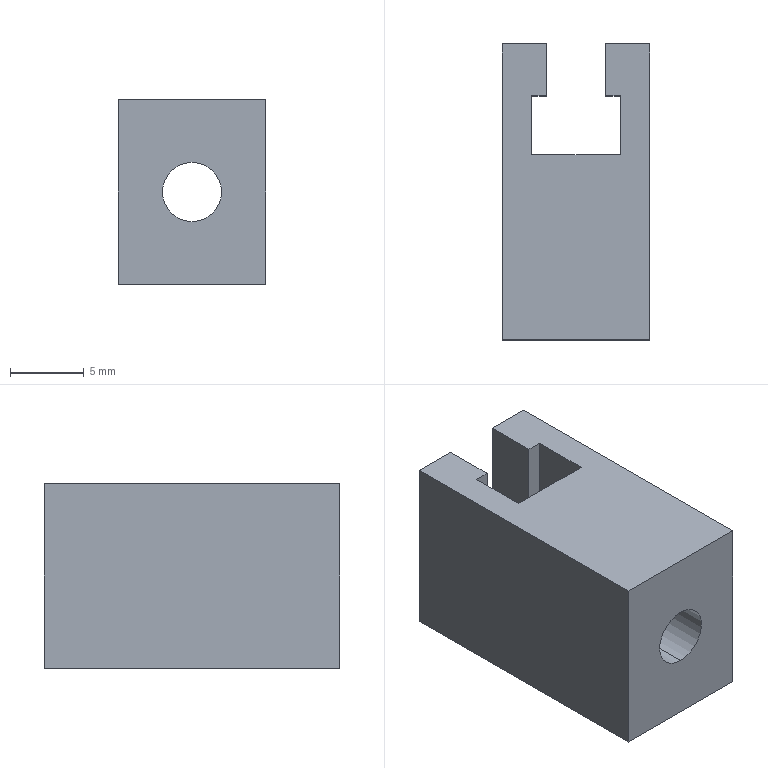Part | STEP file | 1 solid | 16 faces | box 10 x 20 x 12.5 mm | volume 1868 mm3 | plane 14 | cylinder 2 | commonest cylinder face diameters 4 x2
STEP:
#1=CARTESIAN_POINT('',(0.,0.,0.));
#2=DIRECTION('',(0.,0.,1.));
#3=DIRECTION('',(1.,0.,0.));
#4=AXIS2_PLACEMENT_3D('',#1,#2,#3);
#5=CARTESIAN_POINT('',(-38.279,-90.,99.036));
#6=VERTEX_POINT('',#5);
#7=CARTESIAN_POINT('',(-38.279,-77.5,99.036));
#8=VERTEX_POINT('',#7);
#9=CARTESIAN_POINT('',(-38.279,-90.,99.036));
#10=DIRECTION('',(0.,1.,0.));
#11=VECTOR('',#10,1.);
#12=LINE('',#9,#11);
#13=CARTESIAN_POINT('',(-38.279,-90.,97.036));
#14=DIRECTION('',(0.,1.,0.));
#15=DIRECTION('',(0.,0.,1.));
#16=AXIS2_PLACEMENT_3D('',#13,#14,#15);
#17=CYLINDRICAL_SURFACE('',#16,2.);
#18=CARTESIAN_POINT('',(6.283,0.));
#19=DIRECTION('',(0.,1.));
#20=VECTOR('',#19,1.);
#21=LINE('',#18,#20);
#22=(GEOMETRIC_REPRESENTATION_CONTEXT(2)PARAMETRIC_REPRESENTATION_CONTEXT()REPRESENTATION_CONTEXT('',''));
#23=DEFINITIONAL_REPRESENTATION('',(#21),#22);
#24=PCURVE('',#17,#23);
#25=CARTESIAN_POINT('',(-38.279,-90.,97.036));
#26=DIRECTION('',(0.,1.,0.));
#27=DIRECTION('',(0.,0.,1.));
#28=AXIS2_PLACEMENT_3D('',#25,#26,#27);
#29=CYLINDRICAL_SURFACE('',#28,2.);
#30=CARTESIAN_POINT('',(0.,0.));
#31=DIRECTION('',(0.,1.));
#32=VECTOR('',#31,1.);
#33=LINE('',#30,#32);
#34=(GEOMETRIC_REPRESENTATION_CONTEXT(2)PARAMETRIC_REPRESENTATION_CONTEXT()REPRESENTATION_CONTEXT('',''));
#35=DEFINITIONAL_REPRESENTATION('',(#33),#34);
#36=PCURVE('',#29,#35);
#37=SURFACE_CURVE('',#12,(#24,#36),.PCURVE_S1.);
#38=EDGE_CURVE('',#6,#8,#37,.T.);
#39=ORIENTED_EDGE('',*,*,#38,.T.);
#40=CARTESIAN_POINT('',(-38.279,-77.5,95.036));
#41=VERTEX_POINT('',#40);
#42=CARTESIAN_POINT('',(-38.279,-77.5,97.036));
#43=DIRECTION('',(0.,-1.,0.));
#44=DIRECTION('',(0.,0.,-1.));
#45=AXIS2_PLACEMENT_3D('',#42,#43,#44);
#46=CIRCLE('',#45,2.);
#47=CARTESIAN_POINT('',(9.425,12.5));
#48=DIRECTION('',(-1.,0.));
#49=VECTOR('',#48,1.);
#50=LINE('',#47,#49);
#51=(GEOMETRIC_REPRESENTATION_CONTEXT(2)PARAMETRIC_REPRESENTATION_CONTEXT()REPRESENTATION_CONTEXT('',''));
#52=DEFINITIONAL_REPRESENTATION('',(#50),#51);
#53=PCURVE('',#17,#52);
#54=CARTESIAN_POINT('',(-72.862,-77.5,115.03));
#55=DIRECTION('',(0.,-1.,0.));
#56=DIRECTION('',(0.,0.,-1.));
#57=AXIS2_PLACEMENT_3D('',#54,#55,#56);
#58=PLANE('',#57);
#59=CARTESIAN_POINT('',(17.994,34.584));
#60=DIRECTION('',(1.,0.));
#61=AXIS2_PLACEMENT_2D('',#59,#60);
#62=CIRCLE('',#61,2.);
#63=(GEOMETRIC_REPRESENTATION_CONTEXT(2)PARAMETRIC_REPRESENTATION_CONTEXT()REPRESENTATION_CONTEXT('',''));
#64=DEFINITIONAL_REPRESENTATION('',(#62),#63);
#65=PCURVE('',#58,#64);
#66=SURFACE_CURVE('',#46,(#53,#65),.PCURVE_S1.);
#67=EDGE_CURVE('',#8,#41,#66,.T.);
#68=ORIENTED_EDGE('',*,*,#67,.T.);
#69=CARTESIAN_POINT('',(-38.279,-90.,95.036));
#70=VERTEX_POINT('',#69);
#71=CARTESIAN_POINT('',(-38.279,-90.,95.036));
#72=DIRECTION('',(0.,1.,0.));
#73=VECTOR('',#72,1.);
#74=LINE('',#71,#73);
#75=CARTESIAN_POINT('',(3.142,0.));
#76=DIRECTION('',(0.,1.));
#77=VECTOR('',#76,1.);
#78=LINE('',#75,#77);
#79=(GEOMETRIC_REPRESENTATION_CONTEXT(2)PARAMETRIC_REPRESENTATION_CONTEXT()REPRESENTATION_CONTEXT('',''));
#80=DEFINITIONAL_REPRESENTATION('',(#78),#79);
#81=PCURVE('',#17,#80);
#82=CARTESIAN_POINT('',(3.142,0.));
#83=DIRECTION('',(0.,1.));
#84=VECTOR('',#83,1.);
#85=LINE('',#82,#84);
#86=(GEOMETRIC_REPRESENTATION_CONTEXT(2)PARAMETRIC_REPRESENTATION_CONTEXT()REPRESENTATION_CONTEXT('',''));
#87=DEFINITIONAL_REPRESENTATION('',(#85),#86);
#88=PCURVE('',#29,#87);
#89=SURFACE_CURVE('',#74,(#81,#88),.PCURVE_S1.);
#90=EDGE_CURVE('',#70,#41,#89,.T.);
#91=ORIENTED_EDGE('',*,*,#90,.F.);
#92=CARTESIAN_POINT('',(-38.279,-90.,97.036));
#93=DIRECTION('',(0.,1.,0.));
#94=DIRECTION('',(0.,0.,1.));
#95=AXIS2_PLACEMENT_3D('',#92,#93,#94);
#96=CIRCLE('',#95,2.);
#97=CARTESIAN_POINT('',(0.,0.));
#98=DIRECTION('',(1.,0.));
#99=VECTOR('',#98,1.);
#100=LINE('',#97,#99);
#101=(GEOMETRIC_REPRESENTATION_CONTEXT(2)PARAMETRIC_REPRESENTATION_CONTEXT()REPRESENTATION_CONTEXT('',''));
#102=DEFINITIONAL_REPRESENTATION('',(#100),#101);
#103=PCURVE('',#17,#102);
#104=CARTESIAN_POINT('',(-38.279,-90.,90.286));
#105=DIRECTION('',(0.,-1.,0.));
#106=DIRECTION('',(0.,0.,-1.));
#107=AXIS2_PLACEMENT_3D('',#104,#105,#106);
#108=PLANE('',#107);
#109=CARTESIAN_POINT('',(-8.75,0.));
#110=CARTESIAN_POINT('',(-8.75,3.464));
#111=CARTESIAN_POINT('',(-5.75,1.732));
#112=CARTESIAN_POINT('',(-2.75,0.));
#113=CARTESIAN_POINT('',(-5.75,-1.732));
#114=CARTESIAN_POINT('',(-8.75,-3.464));
#115=CARTESIAN_POINT('',(-8.75,0.));
#116=(BOUNDED_CURVE()B_SPLINE_CURVE(2,(#109,#110,#111,#112,#113,#114,#115),.UNSPECIFIED.,.T.,.F.)B_SPLINE_CURVE_WITH_KNOTS((1,2,2,2,2,1),(-2.094,0.,2.094,4.189,6.283,8.378),.UNSPECIFIED.)CURVE()GEOMETRIC_REPRESENTATION_ITEM()RATIONAL_B_SPLINE_CURVE((1.,0.5,1.,0.5,1.,0.5,1.))REPRESENTATION_ITEM(''));
#117=(GEOMETRIC_REPRESENTATION_CONTEXT(2)PARAMETRIC_REPRESENTATION_CONTEXT()REPRESENTATION_CONTEXT('',''));
#118=DEFINITIONAL_REPRESENTATION('',(#116),#117);
#119=PCURVE('',#108,#118);
#120=SURFACE_CURVE('',#96,(#103,#119),.PCURVE_S1.);
#121=EDGE_CURVE('',#70,#6,#120,.T.);
#122=ORIENTED_EDGE('',*,*,#121,.T.);
#123=EDGE_LOOP('',(#39,#68,#91,#122));
#124=FACE_BOUND('',#123,.F.);
#125=ADVANCED_FACE('',(#124),#17,.F.);
#126=CARTESIAN_POINT('',(-41.279,-73.5,103.286));
#127=VERTEX_POINT('',#126);
#128=CARTESIAN_POINT('',(-40.279,-73.5,103.286));
#129=VERTEX_POINT('',#128);
#130=CARTESIAN_POINT('',(-38.279,-73.5,103.286));
#131=DIRECTION('',(1.,0.,0.));
#132=VECTOR('',#131,1.);
#133=LINE('',#130,#132);
#134=CARTESIAN_POINT('',(-38.279,-85.,103.286));
#135=DIRECTION('',(0.,0.,1.));
#136=DIRECTION('',(1.,0.,0.));
#137=AXIS2_PLACEMENT_3D('',#134,#135,#136);
#138=PLANE('',#137);
#139=CARTESIAN_POINT('',(0.,11.5));
#140=DIRECTION('',(1.,0.));
#141=VECTOR('',#140,1.);
#142=LINE('',#139,#141);
#143=(GEOMETRIC_REPRESENTATION_CONTEXT(2)PARAMETRIC_REPRESENTATION_CONTEXT()REPRESENTATION_CONTEXT('',''));
#144=DEFINITIONAL_REPRESENTATION('',(#142),#143);
#145=PCURVE('',#138,#144);
#146=CARTESIAN_POINT('',(-38.279,-73.5,95.192));
#147=DIRECTION('',(0.,-1.,0.));
#148=DIRECTION('',(0.,0.,-1.));
#149=AXIS2_PLACEMENT_3D('',#146,#147,#148);
#150=PLANE('',#149);
#151=CARTESIAN_POINT('',(-8.093,0.));
#152=DIRECTION('',(0.,1.));
#153=VECTOR('',#152,1.);
#154=LINE('',#151,#153);
#155=(GEOMETRIC_REPRESENTATION_CONTEXT(2)PARAMETRIC_REPRESENTATION_CONTEXT()REPRESENTATION_CONTEXT('',''));
#156=DEFINITIONAL_REPRESENTATION('',(#154),#155);
#157=PCURVE('',#150,#156);
#158=SURFACE_CURVE('',#133,(#145,#157),.PCURVE_S1.);
#159=EDGE_CURVE('',#127,#129,#158,.T.);
#160=ORIENTED_EDGE('',*,*,#159,.T.);
#161=CARTESIAN_POINT('',(-40.279,-70.,103.286));
#162=VERTEX_POINT('',#161);
#163=CARTESIAN_POINT('',(-40.279,-85.,103.286));
#164=DIRECTION('',(0.,1.,0.));
#165=VECTOR('',#164,1.);
#166=LINE('',#163,#165);
#167=CARTESIAN_POINT('',(-2.,0.));
#168=DIRECTION('',(0.,1.));
#169=VECTOR('',#168,1.);
#170=LINE('',#167,#169);
#171=(GEOMETRIC_REPRESENTATION_CONTEXT(2)PARAMETRIC_REPRESENTATION_CONTEXT()REPRESENTATION_CONTEXT('',''));
#172=DEFINITIONAL_REPRESENTATION('',(#170),#171);
#173=PCURVE('',#138,#172);
#174=CARTESIAN_POINT('',(-40.279,-38.669,100.65));
#175=DIRECTION('',(1.,0.,0.));
#176=DIRECTION('',(0.,0.,-1.));
#177=AXIS2_PLACEMENT_3D('',#174,#175,#176);
#178=PLANE('',#177);
#179=CARTESIAN_POINT('',(-2.636,-46.331));
#180=DIRECTION('',(0.,1.));
#181=VECTOR('',#180,1.);
#182=LINE('',#179,#181);
#183=(GEOMETRIC_REPRESENTATION_CONTEXT(2)PARAMETRIC_REPRESENTATION_CONTEXT()REPRESENTATION_CONTEXT('',''));
#184=DEFINITIONAL_REPRESENTATION('',(#182),#183);
#185=PCURVE('',#178,#184);
#186=SURFACE_CURVE('',#166,(#173,#185),.PCURVE_S1.);
#187=EDGE_CURVE('',#129,#162,#186,.T.);
#188=ORIENTED_EDGE('',*,*,#187,.T.);
#189=CARTESIAN_POINT('',(-43.279,-70.,103.286));
#190=VERTEX_POINT('',#189);
#191=CARTESIAN_POINT('',(-38.279,-70.,103.286));
#192=DIRECTION('',(1.,0.,0.));
#193=VECTOR('',#192,1.);
#194=LINE('',#191,#193);
#195=CARTESIAN_POINT('',(0.,15.));
#196=DIRECTION('',(1.,0.));
#197=VECTOR('',#196,1.);
#198=LINE('',#195,#197);
#199=(GEOMETRIC_REPRESENTATION_CONTEXT(2)PARAMETRIC_REPRESENTATION_CONTEXT()REPRESENTATION_CONTEXT('',''));
#200=DEFINITIONAL_REPRESENTATION('',(#198),#199);
#201=PCURVE('',#138,#200);
#202=CARTESIAN_POINT('',(-38.279,-70.,90.286));
#203=DIRECTION('',(0.,1.,0.));
#204=DIRECTION('',(0.,0.,1.));
#205=AXIS2_PLACEMENT_3D('',#202,#203,#204);
#206=PLANE('',#205);
#207=CARTESIAN_POINT('',(13.,0.));
#208=DIRECTION('',(0.,1.));
#209=VECTOR('',#208,1.);
#210=LINE('',#207,#209);
#211=(GEOMETRIC_REPRESENTATION_CONTEXT(2)PARAMETRIC_REPRESENTATION_CONTEXT()REPRESENTATION_CONTEXT('',''));
#212=DEFINITIONAL_REPRESENTATION('',(#210),#211);
#213=PCURVE('',#206,#212);
#214=SURFACE_CURVE('',#194,(#201,#213),.PCURVE_S1.);
#215=EDGE_CURVE('',#190,#162,#214,.T.);
#216=ORIENTED_EDGE('',*,*,#215,.F.);
#217=CARTESIAN_POINT('',(-43.279,-90.,103.286));
#218=VERTEX_POINT('',#217);
#219=CARTESIAN_POINT('',(-43.279,-85.,103.286));
#220=DIRECTION('',(0.,1.,0.));
#221=VECTOR('',#220,1.);
#222=LINE('',#219,#221);
#223=CARTESIAN_POINT('',(-5.,0.));
#224=DIRECTION('',(0.,1.));
#225=VECTOR('',#224,1.);
#226=LINE('',#223,#225);
#227=(GEOMETRIC_REPRESENTATION_CONTEXT(2)PARAMETRIC_REPRESENTATION_CONTEXT()REPRESENTATION_CONTEXT('',''));
#228=DEFINITIONAL_REPRESENTATION('',(#226),#227);
#229=PCURVE('',#138,#228);
#230=CARTESIAN_POINT('',(-43.279,-85.,90.286));
#231=DIRECTION('',(-1.,0.,0.));
#232=DIRECTION('',(0.,0.,1.));
#233=AXIS2_PLACEMENT_3D('',#230,#231,#232);
#234=PLANE('',#233);
#235=CARTESIAN_POINT('',(13.,0.));
#236=DIRECTION('',(0.,1.));
#237=VECTOR('',#236,1.);
#238=LINE('',#235,#237);
#239=(GEOMETRIC_REPRESENTATION_CONTEXT(2)PARAMETRIC_REPRESENTATION_CONTEXT()REPRESENTATION_CONTEXT('',''));
#240=DEFINITIONAL_REPRESENTATION('',(#238),#239);
#241=PCURVE('',#234,#240);
#242=SURFACE_CURVE('',#222,(#229,#241),.PCURVE_S1.);
#243=EDGE_CURVE('',#218,#190,#242,.T.);
#244=ORIENTED_EDGE('',*,*,#243,.F.);
#245=CARTESIAN_POINT('',(-33.279,-90.,103.286));
#246=VERTEX_POINT('',#245);
#247=CARTESIAN_POINT('',(-38.279,-90.,103.286));
#248=DIRECTION('',(-1.,0.,0.));
#249=VECTOR('',#248,1.);
#250=LINE('',#247,#249);
#251=CARTESIAN_POINT('',(0.,-5.));
#252=DIRECTION('',(-1.,0.));
#253=VECTOR('',#252,1.);
#254=LINE('',#251,#253);
#255=(GEOMETRIC_REPRESENTATION_CONTEXT(2)PARAMETRIC_REPRESENTATION_CONTEXT()REPRESENTATION_CONTEXT('',''));
#256=DEFINITIONAL_REPRESENTATION('',(#254),#255);
#257=PCURVE('',#138,#256);
#258=CARTESIAN_POINT('',(-13.,0.));
#259=DIRECTION('',(0.,-1.));
#260=VECTOR('',#259,1.);
#261=LINE('',#258,#260);
#262=(GEOMETRIC_REPRESENTATION_CONTEXT(2)PARAMETRIC_REPRESENTATION_CONTEXT()REPRESENTATION_CONTEXT('',''));
#263=DEFINITIONAL_REPRESENTATION('',(#261),#262);
#264=PCURVE('',#108,#263);
#265=SURFACE_CURVE('',#250,(#257,#264),.PCURVE_S1.);
#266=EDGE_CURVE('',#246,#218,#265,.T.);
#267=ORIENTED_EDGE('',*,*,#266,.F.);
#268=CARTESIAN_POINT('',(-33.279,-70.,103.286));
#269=VERTEX_POINT('',#268);
#270=CARTESIAN_POINT('',(-33.279,-85.,103.286));
#271=DIRECTION('',(0.,-1.,0.));
#272=VECTOR('',#271,1.);
#273=LINE('',#270,#272);
#274=CARTESIAN_POINT('',(5.,0.));
#275=DIRECTION('',(0.,-1.));
#276=VECTOR('',#275,1.);
#277=LINE('',#274,#276);
#278=(GEOMETRIC_REPRESENTATION_CONTEXT(2)PARAMETRIC_REPRESENTATION_CONTEXT()REPRESENTATION_CONTEXT('',''));
#279=DEFINITIONAL_REPRESENTATION('',(#277),#278);
#280=PCURVE('',#138,#279);
#281=CARTESIAN_POINT('',(-33.279,-85.,90.286));
#282=DIRECTION('',(1.,0.,0.));
#283=DIRECTION('',(0.,0.,-1.));
#284=AXIS2_PLACEMENT_3D('',#281,#282,#283);
#285=PLANE('',#284);
#286=CARTESIAN_POINT('',(-13.,0.));
#287=DIRECTION('',(0.,-1.));
#288=VECTOR('',#287,1.);
#289=LINE('',#286,#288);
#290=(GEOMETRIC_REPRESENTATION_CONTEXT(2)PARAMETRIC_REPRESENTATION_CONTEXT()REPRESENTATION_CONTEXT('',''));
#291=DEFINITIONAL_REPRESENTATION('',(#289),#290);
#292=PCURVE('',#285,#291);
#293=SURFACE_CURVE('',#273,(#280,#292),.PCURVE_S1.);
#294=EDGE_CURVE('',#269,#246,#293,.T.);
#295=ORIENTED_EDGE('',*,*,#294,.F.);
#296=CARTESIAN_POINT('',(-36.279,-70.,103.286));
#297=VERTEX_POINT('',#296);
#298=CARTESIAN_POINT('',(-38.279,-70.,103.286));
#299=DIRECTION('',(1.,0.,0.));
#300=VECTOR('',#299,1.);
#301=LINE('',#298,#300);
#302=CARTESIAN_POINT('',(0.,15.));
#303=DIRECTION('',(1.,0.));
#304=VECTOR('',#303,1.);
#305=LINE('',#302,#304);
#306=(GEOMETRIC_REPRESENTATION_CONTEXT(2)PARAMETRIC_REPRESENTATION_CONTEXT()REPRESENTATION_CONTEXT('',''));
#307=DEFINITIONAL_REPRESENTATION('',(#305),#306);
#308=PCURVE('',#138,#307);
#309=CARTESIAN_POINT('',(-38.279,-70.,90.286));
#310=DIRECTION('',(0.,1.,0.));
#311=DIRECTION('',(0.,0.,1.));
#312=AXIS2_PLACEMENT_3D('',#309,#310,#311);
#313=PLANE('',#312);
#314=CARTESIAN_POINT('',(13.,0.));
#315=DIRECTION('',(0.,1.));
#316=VECTOR('',#315,1.);
#317=LINE('',#314,#316);
#318=(GEOMETRIC_REPRESENTATION_CONTEXT(2)PARAMETRIC_REPRESENTATION_CONTEXT()REPRESENTATION_CONTEXT('',''));
#319=DEFINITIONAL_REPRESENTATION('',(#317),#318);
#320=PCURVE('',#313,#319);
#321=SURFACE_CURVE('',#301,(#308,#320),.PCURVE_S1.);
#322=EDGE_CURVE('',#297,#269,#321,.T.);
#323=ORIENTED_EDGE('',*,*,#322,.F.);
#324=CARTESIAN_POINT('',(-36.279,-73.5,103.286));
#325=VERTEX_POINT('',#324);
#326=CARTESIAN_POINT('',(-36.279,-85.,103.286));
#327=DIRECTION('',(0.,1.,0.));
#328=VECTOR('',#327,1.);
#329=LINE('',#326,#328);
#330=CARTESIAN_POINT('',(2.,0.));
#331=DIRECTION('',(0.,1.));
#332=VECTOR('',#331,1.);
#333=LINE('',#330,#332);
#334=(GEOMETRIC_REPRESENTATION_CONTEXT(2)PARAMETRIC_REPRESENTATION_CONTEXT()REPRESENTATION_CONTEXT('',''));
#335=DEFINITIONAL_REPRESENTATION('',(#333),#334);
#336=PCURVE('',#138,#335);
#337=CARTESIAN_POINT('',(-36.279,-3.669,115.562));
#338=DIRECTION('',(1.,0.,0.));
#339=DIRECTION('',(0.,0.,-1.));
#340=AXIS2_PLACEMENT_3D('',#337,#338,#339);
#341=PLANE('',#340);
#342=CARTESIAN_POINT('',(12.276,-81.331));
#343=DIRECTION('',(0.,1.));
#344=VECTOR('',#343,1.);
#345=LINE('',#342,#344);
#346=(GEOMETRIC_REPRESENTATION_CONTEXT(2)PARAMETRIC_REPRESENTATION_CONTEXT()REPRESENTATION_CONTEXT('',''));
#347=DEFINITIONAL_REPRESENTATION('',(#345),#346);
#348=PCURVE('',#341,#347);
#349=SURFACE_CURVE('',#329,(#336,#348),.PCURVE_S1.);
#350=EDGE_CURVE('',#325,#297,#349,.T.);
#351=ORIENTED_EDGE('',*,*,#350,.F.);
#352=CARTESIAN_POINT('',(-35.279,-73.5,103.286));
#353=VERTEX_POINT('',#352);
#354=CARTESIAN_POINT('',(-38.279,-73.5,103.286));
#355=DIRECTION('',(1.,0.,0.));
#356=VECTOR('',#355,1.);
#357=LINE('',#354,#356);
#358=CARTESIAN_POINT('',(0.,11.5));
#359=DIRECTION('',(1.,0.));
#360=VECTOR('',#359,1.);
#361=LINE('',#358,#360);
#362=(GEOMETRIC_REPRESENTATION_CONTEXT(2)PARAMETRIC_REPRESENTATION_CONTEXT()REPRESENTATION_CONTEXT('',''));
#363=DEFINITIONAL_REPRESENTATION('',(#361),#362);
#364=PCURVE('',#138,#363);
#365=CARTESIAN_POINT('',(-38.279,-73.5,95.192));
#366=DIRECTION('',(0.,-1.,0.));
#367=DIRECTION('',(0.,0.,-1.));
#368=AXIS2_PLACEMENT_3D('',#365,#366,#367);
#369=PLANE('',#368);
#370=CARTESIAN_POINT('',(-8.093,0.));
#371=DIRECTION('',(0.,1.));
#372=VECTOR('',#371,1.);
#373=LINE('',#370,#372);
#374=(GEOMETRIC_REPRESENTATION_CONTEXT(2)PARAMETRIC_REPRESENTATION_CONTEXT()REPRESENTATION_CONTEXT('',''));
#375=DEFINITIONAL_REPRESENTATION('',(#373),#374);
#376=PCURVE('',#369,#375);
#377=SURFACE_CURVE('',#357,(#364,#376),.PCURVE_S1.);
#378=EDGE_CURVE('',#325,#353,#377,.T.);
#379=ORIENTED_EDGE('',*,*,#378,.T.);
#380=CARTESIAN_POINT('',(-35.279,-77.5,103.286));
#381=VERTEX_POINT('',#380);
#382=CARTESIAN_POINT('',(-35.279,-85.,103.286));
#383=DIRECTION('',(0.,1.,0.));
#384=VECTOR('',#383,1.);
#385=LINE('',#382,#384);
#386=CARTESIAN_POINT('',(3.,0.));
#387=DIRECTION('',(0.,1.));
#388=VECTOR('',#387,1.);
#389=LINE('',#386,#388);
#390=(GEOMETRIC_REPRESENTATION_CONTEXT(2)PARAMETRIC_REPRESENTATION_CONTEXT()REPRESENTATION_CONTEXT('',''));
#391=DEFINITIONAL_REPRESENTATION('',(#389),#390);
#392=PCURVE('',#138,#391);
#393=CARTESIAN_POINT('',(-35.279,-3.669,115.562));
#394=DIRECTION('',(1.,0.,0.));
#395=DIRECTION('',(0.,0.,-1.));
#396=AXIS2_PLACEMENT_3D('',#393,#394,#395);
#397=PLANE('',#396);
#398=CARTESIAN_POINT('',(12.276,-81.331));
#399=DIRECTION('',(0.,1.));
#400=VECTOR('',#399,1.);
#401=LINE('',#398,#400);
#402=(GEOMETRIC_REPRESENTATION_CONTEXT(2)PARAMETRIC_REPRESENTATION_CONTEXT()REPRESENTATION_CONTEXT('',''));
#403=DEFINITIONAL_REPRESENTATION('',(#401),#402);
#404=PCURVE('',#397,#403);
#405=SURFACE_CURVE('',#385,(#392,#404),.PCURVE_S1.);
#406=EDGE_CURVE('',#381,#353,#405,.T.);
#407=ORIENTED_EDGE('',*,*,#406,.F.);
#408=CARTESIAN_POINT('',(-41.279,-77.5,103.286));
#409=VERTEX_POINT('',#408);
#410=CARTESIAN_POINT('',(-38.279,-77.5,103.286));
#411=DIRECTION('',(1.,0.,0.));
#412=VECTOR('',#411,1.);
#413=LINE('',#410,#412);
#414=CARTESIAN_POINT('',(0.,7.5));
#415=DIRECTION('',(1.,0.));
#416=VECTOR('',#415,1.);
#417=LINE('',#414,#416);
#418=(GEOMETRIC_REPRESENTATION_CONTEXT(2)PARAMETRIC_REPRESENTATION_CONTEXT()REPRESENTATION_CONTEXT('',''));
#419=DEFINITIONAL_REPRESENTATION('',(#417),#418);
#420=PCURVE('',#138,#419);
#421=CARTESIAN_POINT('',(11.744,34.584));
#422=DIRECTION('',(0.,1.));
#423=VECTOR('',#422,1.);
#424=LINE('',#421,#423);
#425=(GEOMETRIC_REPRESENTATION_CONTEXT(2)PARAMETRIC_REPRESENTATION_CONTEXT()REPRESENTATION_CONTEXT('',''));
#426=DEFINITIONAL_REPRESENTATION('',(#424),#425);
#427=PCURVE('',#58,#426);
#428=SURFACE_CURVE('',#413,(#420,#427),.PCURVE_S1.);
#429=EDGE_CURVE('',#409,#381,#428,.T.);
#430=ORIENTED_EDGE('',*,*,#429,.F.);
#431=CARTESIAN_POINT('',(-41.279,-85.,103.286));
#432=DIRECTION('',(0.,1.,0.));
#433=VECTOR('',#432,1.);
#434=LINE('',#431,#433);
#435=CARTESIAN_POINT('',(-3.,0.));
#436=DIRECTION('',(0.,1.));
#437=VECTOR('',#436,1.);
#438=LINE('',#435,#437);
#439=(GEOMETRIC_REPRESENTATION_CONTEXT(2)PARAMETRIC_REPRESENTATION_CONTEXT()REPRESENTATION_CONTEXT('',''));
#440=DEFINITIONAL_REPRESENTATION('',(#438),#439);
#441=PCURVE('',#138,#440);
#442=CARTESIAN_POINT('',(-41.279,-38.669,100.65));
#443=DIRECTION('',(1.,0.,0.));
#444=DIRECTION('',(0.,0.,-1.));
#445=AXIS2_PLACEMENT_3D('',#442,#443,#444);
#446=PLANE('',#445);
#447=CARTESIAN_POINT('',(-2.636,-46.331));
#448=DIRECTION('',(0.,1.));
#449=VECTOR('',#448,1.);
#450=LINE('',#447,#449);
#451=(GEOMETRIC_REPRESENTATION_CONTEXT(2)PARAMETRIC_REPRESENTATION_CONTEXT()REPRESENTATION_CONTEXT('',''));
#452=DEFINITIONAL_REPRESENTATION('',(#450),#451);
#453=PCURVE('',#446,#452);
#454=SURFACE_CURVE('',#434,(#441,#453),.PCURVE_S1.);
#455=EDGE_CURVE('',#409,#127,#454,.T.);
#456=ORIENTED_EDGE('',*,*,#455,.T.);
#457=EDGE_LOOP('',(#160,#188,#216,#244,#267,#295,#323,#351,#379,#407,#430,#456));
#458=FACE_BOUND('',#457,.T.);
#459=ADVANCED_FACE('',(#458),#138,.T.);
#460=ORIENTED_EDGE('',*,*,#215,.T.);
#461=CARTESIAN_POINT('',(-40.279,-70.,90.786));
#462=VERTEX_POINT('',#461);
#463=CARTESIAN_POINT('',(-40.279,-70.,90.286));
#464=DIRECTION('',(0.,0.,-1.));
#465=VECTOR('',#464,1.);
#466=LINE('',#463,#465);
#467=CARTESIAN_POINT('',(0.,-2.));
#468=DIRECTION('',(-1.,0.));
#469=VECTOR('',#468,1.);
#470=LINE('',#467,#469);
#471=(GEOMETRIC_REPRESENTATION_CONTEXT(2)PARAMETRIC_REPRESENTATION_CONTEXT()REPRESENTATION_CONTEXT('',''));
#472=DEFINITIONAL_REPRESENTATION('',(#470),#471);
#473=PCURVE('',#206,#472);
#474=CARTESIAN_POINT('',(10.364,-31.331));
#475=DIRECTION('',(1.,0.));
#476=VECTOR('',#475,1.);
#477=LINE('',#474,#476);
#478=(GEOMETRIC_REPRESENTATION_CONTEXT(2)PARAMETRIC_REPRESENTATION_CONTEXT()REPRESENTATION_CONTEXT('',''));
#479=DEFINITIONAL_REPRESENTATION('',(#477),#478);
#480=PCURVE('',#178,#479);
#481=SURFACE_CURVE('',#466,(#473,#480),.PCURVE_S1.);
#482=EDGE_CURVE('',#162,#462,#481,.T.);
#483=ORIENTED_EDGE('',*,*,#482,.T.);
#484=CARTESIAN_POINT('',(-43.279,-70.,90.786));
#485=VERTEX_POINT('',#484);
#486=CARTESIAN_POINT('',(-38.279,-70.,90.786));
#487=DIRECTION('',(-1.,0.,0.));
#488=VECTOR('',#487,1.);
#489=LINE('',#486,#488);
#490=CARTESIAN_POINT('',(0.5,0.));
#491=DIRECTION('',(0.,-1.));
#492=VECTOR('',#491,1.);
#493=LINE('',#490,#492);
#494=(GEOMETRIC_REPRESENTATION_CONTEXT(2)PARAMETRIC_REPRESENTATION_CONTEXT()REPRESENTATION_CONTEXT('',''));
#495=DEFINITIONAL_REPRESENTATION('',(#493),#494);
#496=PCURVE('',#206,#495);
#497=CARTESIAN_POINT('',(-38.279,-85.,90.786));
#498=DIRECTION('',(0.,0.,-1.));
#499=DIRECTION('',(-1.,0.,0.));
#500=AXIS2_PLACEMENT_3D('',#497,#498,#499);
#501=PLANE('',#500);
#502=CARTESIAN_POINT('',(0.,15.));
#503=DIRECTION('',(1.,0.));
#504=VECTOR('',#503,1.);
#505=LINE('',#502,#504);
#506=(GEOMETRIC_REPRESENTATION_CONTEXT(2)PARAMETRIC_REPRESENTATION_CONTEXT()REPRESENTATION_CONTEXT('',''));
#507=DEFINITIONAL_REPRESENTATION('',(#505),#506);
#508=PCURVE('',#501,#507);
#509=SURFACE_CURVE('',#489,(#496,#508),.PCURVE_S1.);
#510=EDGE_CURVE('',#462,#485,#509,.T.);
#511=ORIENTED_EDGE('',*,*,#510,.T.);
#512=CARTESIAN_POINT('',(-43.279,-70.,90.286));
#513=DIRECTION('',(0.,0.,1.));
#514=VECTOR('',#513,1.);
#515=LINE('',#512,#514);
#516=CARTESIAN_POINT('',(0.,-5.));
#517=DIRECTION('',(1.,0.));
#518=VECTOR('',#517,1.);
#519=LINE('',#516,#518);
#520=(GEOMETRIC_REPRESENTATION_CONTEXT(2)PARAMETRIC_REPRESENTATION_CONTEXT()REPRESENTATION_CONTEXT('',''));
#521=DEFINITIONAL_REPRESENTATION('',(#519),#520);
#522=PCURVE('',#206,#521);
#523=CARTESIAN_POINT('',(0.,15.));
#524=DIRECTION('',(1.,0.));
#525=VECTOR('',#524,1.);
#526=LINE('',#523,#525);
#527=(GEOMETRIC_REPRESENTATION_CONTEXT(2)PARAMETRIC_REPRESENTATION_CONTEXT()REPRESENTATION_CONTEXT('',''));
#528=DEFINITIONAL_REPRESENTATION('',(#526),#527);
#529=PCURVE('',#234,#528);
#530=SURFACE_CURVE('',#515,(#522,#529),.PCURVE_S1.);
#531=EDGE_CURVE('',#485,#190,#530,.T.);
#532=ORIENTED_EDGE('',*,*,#531,.T.);
#533=EDGE_LOOP('',(#460,#483,#511,#532));
#534=FACE_BOUND('',#533,.T.);
#535=ADVANCED_FACE('',(#534),#206,.T.);
#536=ORIENTED_EDGE('',*,*,#510,.F.);
#537=CARTESIAN_POINT('',(-40.279,-73.5,90.786));
#538=VERTEX_POINT('',#537);
#539=CARTESIAN_POINT('',(-40.279,-85.,90.786));
#540=DIRECTION('',(0.,-1.,0.));
#541=VECTOR('',#540,1.);
#542=LINE('',#539,#541);
#543=CARTESIAN_POINT('',(2.,0.));
#544=DIRECTION('',(0.,-1.));
#545=VECTOR('',#544,1.);
#546=LINE('',#543,#545);
#547=(GEOMETRIC_REPRESENTATION_CONTEXT(2)PARAMETRIC_REPRESENTATION_CONTEXT()REPRESENTATION_CONTEXT('',''));
#548=DEFINITIONAL_REPRESENTATION('',(#546),#547);
#549=PCURVE('',#501,#548);
#550=CARTESIAN_POINT('',(9.864,-46.331));
#551=DIRECTION('',(0.,-1.));
#552=VECTOR('',#551,1.);
#553=LINE('',#550,#552);
#554=(GEOMETRIC_REPRESENTATION_CONTEXT(2)PARAMETRIC_REPRESENTATION_CONTEXT()REPRESENTATION_CONTEXT('',''));
#555=DEFINITIONAL_REPRESENTATION('',(#553),#554);
#556=PCURVE('',#178,#555);
#557=SURFACE_CURVE('',#542,(#549,#556),.PCURVE_S1.);
#558=EDGE_CURVE('',#462,#538,#557,.T.);
#559=ORIENTED_EDGE('',*,*,#558,.T.);
#560=CARTESIAN_POINT('',(-41.279,-73.5,90.786));
#561=VERTEX_POINT('',#560);
#562=CARTESIAN_POINT('',(-38.279,-73.5,90.786));
#563=DIRECTION('',(-1.,0.,0.));
#564=VECTOR('',#563,1.);
#565=LINE('',#562,#564);
#566=CARTESIAN_POINT('',(0.,11.5));
#567=DIRECTION('',(1.,0.));
#568=VECTOR('',#567,1.);
#569=LINE('',#566,#568);
#570=(GEOMETRIC_REPRESENTATION_CONTEXT(2)PARAMETRIC_REPRESENTATION_CONTEXT()REPRESENTATION_CONTEXT('',''));
#571=DEFINITIONAL_REPRESENTATION('',(#569),#570);
#572=PCURVE('',#501,#571);
#573=CARTESIAN_POINT('',(4.407,0.));
#574=DIRECTION('',(0.,-1.));
#575=VECTOR('',#574,1.);
#576=LINE('',#573,#575);
#577=(GEOMETRIC_REPRESENTATION_CONTEXT(2)PARAMETRIC_REPRESENTATION_CONTEXT()REPRESENTATION_CONTEXT('',''));
#578=DEFINITIONAL_REPRESENTATION('',(#576),#577);
#579=PCURVE('',#150,#578);
#580=SURFACE_CURVE('',#565,(#572,#579),.PCURVE_S1.);
#581=EDGE_CURVE('',#538,#561,#580,.T.);
#582=ORIENTED_EDGE('',*,*,#581,.T.);
#583=CARTESIAN_POINT('',(-41.279,-77.5,90.786));
#584=VERTEX_POINT('',#583);
#585=CARTESIAN_POINT('',(-41.279,-85.,90.786));
#586=DIRECTION('',(0.,-1.,0.));
#587=VECTOR('',#586,1.);
#588=LINE('',#585,#587);
#589=CARTESIAN_POINT('',(3.,0.));
#590=DIRECTION('',(0.,-1.));
#591=VECTOR('',#590,1.);
#592=LINE('',#589,#591);
#593=(GEOMETRIC_REPRESENTATION_CONTEXT(2)PARAMETRIC_REPRESENTATION_CONTEXT()REPRESENTATION_CONTEXT('',''));
#594=DEFINITIONAL_REPRESENTATION('',(#592),#593);
#595=PCURVE('',#501,#594);
#596=CARTESIAN_POINT('',(9.864,-46.331));
#597=DIRECTION('',(0.,-1.));
#598=VECTOR('',#597,1.);
#599=LINE('',#596,#598);
#600=(GEOMETRIC_REPRESENTATION_CONTEXT(2)PARAMETRIC_REPRESENTATION_CONTEXT()REPRESENTATION_CONTEXT('',''));
#601=DEFINITIONAL_REPRESENTATION('',(#599),#600);
#602=PCURVE('',#446,#601);
#603=SURFACE_CURVE('',#588,(#595,#602),.PCURVE_S1.);
#604=EDGE_CURVE('',#561,#584,#603,.T.);
#605=ORIENTED_EDGE('',*,*,#604,.T.);
#606=CARTESIAN_POINT('',(-35.279,-77.5,90.786));
#607=VERTEX_POINT('',#606);
#608=CARTESIAN_POINT('',(-38.279,-77.5,90.786));
#609=DIRECTION('',(-1.,0.,0.));
#610=VECTOR('',#609,1.);
#611=LINE('',#608,#610);
#612=CARTESIAN_POINT('',(0.,7.5));
#613=DIRECTION('',(1.,0.));
#614=VECTOR('',#613,1.);
#615=LINE('',#612,#614);
#616=(GEOMETRIC_REPRESENTATION_CONTEXT(2)PARAMETRIC_REPRESENTATION_CONTEXT()REPRESENTATION_CONTEXT('',''));
#617=DEFINITIONAL_REPRESENTATION('',(#615),#616);
#618=PCURVE('',#501,#617);
#619=CARTESIAN_POINT('',(24.244,34.584));
#620=DIRECTION('',(0.,-1.));
#621=VECTOR('',#620,1.);
#622=LINE('',#619,#621);
#623=(GEOMETRIC_REPRESENTATION_CONTEXT(2)PARAMETRIC_REPRESENTATION_CONTEXT()REPRESENTATION_CONTEXT('',''));
#624=DEFINITIONAL_REPRESENTATION('',(#622),#623);
#625=PCURVE('',#58,#624);
#626=SURFACE_CURVE('',#611,(#618,#625),.PCURVE_S1.);
#627=EDGE_CURVE('',#607,#584,#626,.T.);
#628=ORIENTED_EDGE('',*,*,#627,.F.);
#629=CARTESIAN_POINT('',(-35.279,-73.5,90.786));
#630=VERTEX_POINT('',#629);
#631=CARTESIAN_POINT('',(-35.279,-85.,90.786));
#632=DIRECTION('',(0.,-1.,0.));
#633=VECTOR('',#632,1.);
#634=LINE('',#631,#633);
#635=CARTESIAN_POINT('',(-3.,0.));
#636=DIRECTION('',(0.,-1.));
#637=VECTOR('',#636,1.);
#638=LINE('',#635,#637);
#639=(GEOMETRIC_REPRESENTATION_CONTEXT(2)PARAMETRIC_REPRESENTATION_CONTEXT()REPRESENTATION_CONTEXT('',''));
#640=DEFINITIONAL_REPRESENTATION('',(#638),#639);
#641=PCURVE('',#501,#640);
#642=CARTESIAN_POINT('',(24.776,-81.331));
#643=DIRECTION('',(0.,-1.));
#644=VECTOR('',#643,1.);
#645=LINE('',#642,#644);
#646=(GEOMETRIC_REPRESENTATION_CONTEXT(2)PARAMETRIC_REPRESENTATION_CONTEXT()REPRESENTATION_CONTEXT('',''));
#647=DEFINITIONAL_REPRESENTATION('',(#645),#646);
#648=PCURVE('',#397,#647);
#649=SURFACE_CURVE('',#634,(#641,#648),.PCURVE_S1.);
#650=EDGE_CURVE('',#630,#607,#649,.T.);
#651=ORIENTED_EDGE('',*,*,#650,.F.);
#652=CARTESIAN_POINT('',(-36.279,-73.5,90.786));
#653=VERTEX_POINT('',#652);
#654=CARTESIAN_POINT('',(-38.279,-73.5,90.786));
#655=DIRECTION('',(-1.,0.,0.));
#656=VECTOR('',#655,1.);
#657=LINE('',#654,#656);
#658=CARTESIAN_POINT('',(0.,11.5));
#659=DIRECTION('',(1.,0.));
#660=VECTOR('',#659,1.);
#661=LINE('',#658,#660);
#662=(GEOMETRIC_REPRESENTATION_CONTEXT(2)PARAMETRIC_REPRESENTATION_CONTEXT()REPRESENTATION_CONTEXT('',''));
#663=DEFINITIONAL_REPRESENTATION('',(#661),#662);
#664=PCURVE('',#501,#663);
#665=CARTESIAN_POINT('',(4.407,0.));
#666=DIRECTION('',(0.,-1.));
#667=VECTOR('',#666,1.);
#668=LINE('',#665,#667);
#669=(GEOMETRIC_REPRESENTATION_CONTEXT(2)PARAMETRIC_REPRESENTATION_CONTEXT()REPRESENTATION_CONTEXT('',''));
#670=DEFINITIONAL_REPRESENTATION('',(#668),#669);
#671=PCURVE('',#369,#670);
#672=SURFACE_CURVE('',#657,(#664,#671),.PCURVE_S1.);
#673=EDGE_CURVE('',#630,#653,#672,.T.);
#674=ORIENTED_EDGE('',*,*,#673,.T.);
#675=CARTESIAN_POINT('',(-36.279,-70.,90.786));
#676=VERTEX_POINT('',#675);
#677=CARTESIAN_POINT('',(-36.279,-85.,90.786));
#678=DIRECTION('',(0.,-1.,0.));
#679=VECTOR('',#678,1.);
#680=LINE('',#677,#679);
#681=CARTESIAN_POINT('',(-2.,0.));
#682=DIRECTION('',(0.,-1.));
#683=VECTOR('',#682,1.);
#684=LINE('',#681,#683);
#685=(GEOMETRIC_REPRESENTATION_CONTEXT(2)PARAMETRIC_REPRESENTATION_CONTEXT()REPRESENTATION_CONTEXT('',''));
#686=DEFINITIONAL_REPRESENTATION('',(#684),#685);
#687=PCURVE('',#501,#686);
#688=CARTESIAN_POINT('',(24.776,-81.331));
#689=DIRECTION('',(0.,-1.));
#690=VECTOR('',#689,1.);
#691=LINE('',#688,#690);
#692=(GEOMETRIC_REPRESENTATION_CONTEXT(2)PARAMETRIC_REPRESENTATION_CONTEXT()REPRESENTATION_CONTEXT('',''));
#693=DEFINITIONAL_REPRESENTATION('',(#691),#692);
#694=PCURVE('',#341,#693);
#695=SURFACE_CURVE('',#680,(#687,#694),.PCURVE_S1.);
#696=EDGE_CURVE('',#676,#653,#695,.T.);
#697=ORIENTED_EDGE('',*,*,#696,.F.);
#698=CARTESIAN_POINT('',(-33.279,-70.,90.786));
#699=VERTEX_POINT('',#698);
#700=CARTESIAN_POINT('',(-38.279,-70.,90.786));
#701=DIRECTION('',(-1.,0.,0.));
#702=VECTOR('',#701,1.);
#703=LINE('',#700,#702);
#704=CARTESIAN_POINT('',(0.,15.));
#705=DIRECTION('',(1.,0.));
#706=VECTOR('',#705,1.);
#707=LINE('',#704,#706);
#708=(GEOMETRIC_REPRESENTATION_CONTEXT(2)PARAMETRIC_REPRESENTATION_CONTEXT()REPRESENTATION_CONTEXT('',''));
#709=DEFINITIONAL_REPRESENTATION('',(#707),#708);
#710=PCURVE('',#501,#709);
#711=CARTESIAN_POINT('',(0.5,0.));
#712=DIRECTION('',(0.,-1.));
#713=VECTOR('',#712,1.);
#714=LINE('',#711,#713);
#715=(GEOMETRIC_REPRESENTATION_CONTEXT(2)PARAMETRIC_REPRESENTATION_CONTEXT()REPRESENTATION_CONTEXT('',''));
#716=DEFINITIONAL_REPRESENTATION('',(#714),#715);
#717=PCURVE('',#313,#716);
#718=SURFACE_CURVE('',#703,(#710,#717),.PCURVE_S1.);
#719=EDGE_CURVE('',#699,#676,#718,.T.);
#720=ORIENTED_EDGE('',*,*,#719,.F.);
#721=CARTESIAN_POINT('',(-33.279,-90.,90.786));
#722=VERTEX_POINT('',#721);
#723=CARTESIAN_POINT('',(-33.279,-85.,90.786));
#724=DIRECTION('',(0.,1.,0.));
#725=VECTOR('',#724,1.);
#726=LINE('',#723,#725);
#727=CARTESIAN_POINT('',(-5.,0.));
#728=DIRECTION('',(0.,1.));
#729=VECTOR('',#728,1.);
#730=LINE('',#727,#729);
#731=(GEOMETRIC_REPRESENTATION_CONTEXT(2)PARAMETRIC_REPRESENTATION_CONTEXT()REPRESENTATION_CONTEXT('',''));
#732=DEFINITIONAL_REPRESENTATION('',(#730),#731);
#733=PCURVE('',#501,#732);
#734=CARTESIAN_POINT('',(-0.5,0.));
#735=DIRECTION('',(0.,1.));
#736=VECTOR('',#735,1.);
#737=LINE('',#734,#736);
#738=(GEOMETRIC_REPRESENTATION_CONTEXT(2)PARAMETRIC_REPRESENTATION_CONTEXT()REPRESENTATION_CONTEXT('',''));
#739=DEFINITIONAL_REPRESENTATION('',(#737),#738);
#740=PCURVE('',#285,#739);
#741=SURFACE_CURVE('',#726,(#733,#740),.PCURVE_S1.);
#742=EDGE_CURVE('',#722,#699,#741,.T.);
#743=ORIENTED_EDGE('',*,*,#742,.F.);
#744=CARTESIAN_POINT('',(-43.279,-90.,90.786));
#745=VERTEX_POINT('',#744);
#746=CARTESIAN_POINT('',(-38.279,-90.,90.786));
#747=DIRECTION('',(1.,0.,0.));
#748=VECTOR('',#747,1.);
#749=LINE('',#746,#748);
#750=CARTESIAN_POINT('',(0.,-5.));
#751=DIRECTION('',(-1.,0.));
#752=VECTOR('',#751,1.);
#753=LINE('',#750,#752);
#754=(GEOMETRIC_REPRESENTATION_CONTEXT(2)PARAMETRIC_REPRESENTATION_CONTEXT()REPRESENTATION_CONTEXT('',''));
#755=DEFINITIONAL_REPRESENTATION('',(#753),#754);
#756=PCURVE('',#501,#755);
#757=CARTESIAN_POINT('',(-0.5,0.));
#758=DIRECTION('',(0.,1.));
#759=VECTOR('',#758,1.);
#760=LINE('',#757,#759);
#761=(GEOMETRIC_REPRESENTATION_CONTEXT(2)PARAMETRIC_REPRESENTATION_CONTEXT()REPRESENTATION_CONTEXT('',''));
#762=DEFINITIONAL_REPRESENTATION('',(#760),#761);
#763=PCURVE('',#108,#762);
#764=SURFACE_CURVE('',#749,(#756,#763),.PCURVE_S1.);
#765=EDGE_CURVE('',#745,#722,#764,.T.);
#766=ORIENTED_EDGE('',*,*,#765,.F.);
#767=CARTESIAN_POINT('',(-43.279,-85.,90.786));
#768=DIRECTION('',(0.,-1.,0.));
#769=VECTOR('',#768,1.);
#770=LINE('',#767,#769);
#771=CARTESIAN_POINT('',(5.,0.));
#772=DIRECTION('',(0.,-1.));
#773=VECTOR('',#772,1.);
#774=LINE('',#771,#773);
#775=(GEOMETRIC_REPRESENTATION_CONTEXT(2)PARAMETRIC_REPRESENTATION_CONTEXT()REPRESENTATION_CONTEXT('',''));
#776=DEFINITIONAL_REPRESENTATION('',(#774),#775);
#777=PCURVE('',#501,#776);
#778=CARTESIAN_POINT('',(0.5,0.));
#779=DIRECTION('',(0.,-1.));
#780=VECTOR('',#779,1.);
#781=LINE('',#778,#780);
#782=(GEOMETRIC_REPRESENTATION_CONTEXT(2)PARAMETRIC_REPRESENTATION_CONTEXT()REPRESENTATION_CONTEXT('',''));
#783=DEFINITIONAL_REPRESENTATION('',(#781),#782);
#784=PCURVE('',#234,#783);
#785=SURFACE_CURVE('',#770,(#777,#784),.PCURVE_S1.);
#786=EDGE_CURVE('',#485,#745,#785,.T.);
#787=ORIENTED_EDGE('',*,*,#786,.F.);
#788=EDGE_LOOP('',(#536,#559,#582,#605,#628,#651,#674,#697,#720,#743,#766,#787));
#789=FACE_BOUND('',#788,.T.);
#790=ADVANCED_FACE('',(#789),#501,.T.);
#791=CARTESIAN_POINT('',(-38.279,-90.,97.036));
#792=DIRECTION('',(0.,1.,0.));
#793=DIRECTION('',(0.,0.,1.));
#794=AXIS2_PLACEMENT_3D('',#791,#792,#793);
#795=CIRCLE('',#794,2.);
#796=CARTESIAN_POINT('',(-8.75,0.));
#797=CARTESIAN_POINT('',(-8.75,3.464));
#798=CARTESIAN_POINT('',(-5.75,1.732));
#799=CARTESIAN_POINT('',(-2.75,0.));
#800=CARTESIAN_POINT('',(-5.75,-1.732));
#801=CARTESIAN_POINT('',(-8.75,-3.464));
#802=CARTESIAN_POINT('',(-8.75,0.));
#803=(BOUNDED_CURVE()B_SPLINE_CURVE(2,(#796,#797,#798,#799,#800,#801,#802),.UNSPECIFIED.,.T.,.F.)B_SPLINE_CURVE_WITH_KNOTS((1,2,2,2,2,1),(-2.094,0.,2.094,4.189,6.283,8.378),.UNSPECIFIED.)CURVE()GEOMETRIC_REPRESENTATION_ITEM()RATIONAL_B_SPLINE_CURVE((1.,0.5,1.,0.5,1.,0.5,1.))REPRESENTATION_ITEM(''));
#804=(GEOMETRIC_REPRESENTATION_CONTEXT(2)PARAMETRIC_REPRESENTATION_CONTEXT()REPRESENTATION_CONTEXT('',''));
#805=DEFINITIONAL_REPRESENTATION('',(#803),#804);
#806=PCURVE('',#108,#805);
#807=CARTESIAN_POINT('',(0.,0.));
#808=DIRECTION('',(1.,0.));
#809=VECTOR('',#808,1.);
#810=LINE('',#807,#809);
#811=(GEOMETRIC_REPRESENTATION_CONTEXT(2)PARAMETRIC_REPRESENTATION_CONTEXT()REPRESENTATION_CONTEXT('',''));
#812=DEFINITIONAL_REPRESENTATION('',(#810),#811);
#813=PCURVE('',#29,#812);
#814=SURFACE_CURVE('',#795,(#806,#813),.PCURVE_S1.);
#815=EDGE_CURVE('',#6,#70,#814,.T.);
#816=ORIENTED_EDGE('',*,*,#815,.T.);
#817=ORIENTED_EDGE('',*,*,#121,.T.);
#818=EDGE_LOOP('',(#816,#817));
#819=FACE_BOUND('',#818,.T.);
#820=CARTESIAN_POINT('',(-33.279,-90.,90.286));
#821=DIRECTION('',(0.,0.,1.));
#822=VECTOR('',#821,1.);
#823=LINE('',#820,#822);
#824=CARTESIAN_POINT('',(0.,5.));
#825=DIRECTION('',(-1.,0.));
#826=VECTOR('',#825,1.);
#827=LINE('',#824,#826);
#828=(GEOMETRIC_REPRESENTATION_CONTEXT(2)PARAMETRIC_REPRESENTATION_CONTEXT()REPRESENTATION_CONTEXT('',''));
#829=DEFINITIONAL_REPRESENTATION('',(#827),#828);
#830=PCURVE('',#108,#829);
#831=CARTESIAN_POINT('',(0.,-5.));
#832=DIRECTION('',(-1.,0.));
#833=VECTOR('',#832,1.);
#834=LINE('',#831,#833);
#835=(GEOMETRIC_REPRESENTATION_CONTEXT(2)PARAMETRIC_REPRESENTATION_CONTEXT()REPRESENTATION_CONTEXT('',''));
#836=DEFINITIONAL_REPRESENTATION('',(#834),#835);
#837=PCURVE('',#285,#836);
#838=SURFACE_CURVE('',#823,(#830,#837),.PCURVE_S1.);
#839=EDGE_CURVE('',#722,#246,#838,.T.);
#840=ORIENTED_EDGE('',*,*,#839,.T.);
#841=ORIENTED_EDGE('',*,*,#266,.T.);
#842=CARTESIAN_POINT('',(-43.279,-90.,90.286));
#843=DIRECTION('',(0.,0.,1.));
#844=VECTOR('',#843,1.);
#845=LINE('',#842,#844);
#846=CARTESIAN_POINT('',(0.,-5.));
#847=DIRECTION('',(-1.,0.));
#848=VECTOR('',#847,1.);
#849=LINE('',#846,#848);
#850=(GEOMETRIC_REPRESENTATION_CONTEXT(2)PARAMETRIC_REPRESENTATION_CONTEXT()REPRESENTATION_CONTEXT('',''));
#851=DEFINITIONAL_REPRESENTATION('',(#849),#850);
#852=PCURVE('',#108,#851);
#853=CARTESIAN_POINT('',(0.,-5.));
#854=DIRECTION('',(1.,0.));
#855=VECTOR('',#854,1.);
#856=LINE('',#853,#855);
#857=(GEOMETRIC_REPRESENTATION_CONTEXT(2)PARAMETRIC_REPRESENTATION_CONTEXT()REPRESENTATION_CONTEXT('',''));
#858=DEFINITIONAL_REPRESENTATION('',(#856),#857);
#859=PCURVE('',#234,#858);
#860=SURFACE_CURVE('',#845,(#852,#859),.PCURVE_S1.);
#861=EDGE_CURVE('',#745,#218,#860,.T.);
#862=ORIENTED_EDGE('',*,*,#861,.F.);
#863=ORIENTED_EDGE('',*,*,#765,.T.);
#864=EDGE_LOOP('',(#840,#841,#862,#863));
#865=FACE_BOUND('',#864,.T.);
#866=ADVANCED_FACE('',(#819,#865),#108,.T.);
#867=ORIENTED_EDGE('',*,*,#861,.T.);
#868=ORIENTED_EDGE('',*,*,#243,.T.);
#869=ORIENTED_EDGE('',*,*,#531,.F.);
#870=ORIENTED_EDGE('',*,*,#786,.T.);
#871=EDGE_LOOP('',(#867,#868,#869,#870));
#872=FACE_BOUND('',#871,.T.);
#873=ADVANCED_FACE('',(#872),#234,.T.);
#874=CARTESIAN_POINT('',(-36.279,-70.,90.286));
#875=DIRECTION('',(0.,0.,-1.));
#876=VECTOR('',#875,1.);
#877=LINE('',#874,#876);
#878=CARTESIAN_POINT('',(0.,2.));
#879=DIRECTION('',(-1.,0.));
#880=VECTOR('',#879,1.);
#881=LINE('',#878,#880);
#882=(GEOMETRIC_REPRESENTATION_CONTEXT(2)PARAMETRIC_REPRESENTATION_CONTEXT()REPRESENTATION_CONTEXT('',''));
#883=DEFINITIONAL_REPRESENTATION('',(#881),#882);
#884=PCURVE('',#313,#883);
#885=CARTESIAN_POINT('',(25.276,-66.331));
#886=DIRECTION('',(1.,0.));
#887=VECTOR('',#886,1.);
#888=LINE('',#885,#887);
#889=(GEOMETRIC_REPRESENTATION_CONTEXT(2)PARAMETRIC_REPRESENTATION_CONTEXT()REPRESENTATION_CONTEXT('',''));
#890=DEFINITIONAL_REPRESENTATION('',(#888),#889);
#891=PCURVE('',#341,#890);
#892=SURFACE_CURVE('',#877,(#884,#891),.PCURVE_S1.);
#893=EDGE_CURVE('',#297,#676,#892,.T.);
#894=ORIENTED_EDGE('',*,*,#893,.F.);
#895=ORIENTED_EDGE('',*,*,#322,.T.);
#896=CARTESIAN_POINT('',(-33.279,-70.,90.286));
#897=DIRECTION('',(0.,0.,1.));
#898=VECTOR('',#897,1.);
#899=LINE('',#896,#898);
#900=CARTESIAN_POINT('',(0.,5.));
#901=DIRECTION('',(1.,0.));
#902=VECTOR('',#901,1.);
#903=LINE('',#900,#902);
#904=(GEOMETRIC_REPRESENTATION_CONTEXT(2)PARAMETRIC_REPRESENTATION_CONTEXT()REPRESENTATION_CONTEXT('',''));
#905=DEFINITIONAL_REPRESENTATION('',(#903),#904);
#906=PCURVE('',#313,#905);
#907=CARTESIAN_POINT('',(0.,15.));
#908=DIRECTION('',(-1.,0.));
#909=VECTOR('',#908,1.);
#910=LINE('',#907,#909);
#911=(GEOMETRIC_REPRESENTATION_CONTEXT(2)PARAMETRIC_REPRESENTATION_CONTEXT()REPRESENTATION_CONTEXT('',''));
#912=DEFINITIONAL_REPRESENTATION('',(#910),#911);
#913=PCURVE('',#285,#912);
#914=SURFACE_CURVE('',#899,(#906,#913),.PCURVE_S1.);
#915=EDGE_CURVE('',#699,#269,#914,.T.);
#916=ORIENTED_EDGE('',*,*,#915,.F.);
#917=ORIENTED_EDGE('',*,*,#719,.T.);
#918=EDGE_LOOP('',(#894,#895,#916,#917));
#919=FACE_BOUND('',#918,.T.);
#920=ADVANCED_FACE('',(#919),#313,.T.);
#921=ORIENTED_EDGE('',*,*,#742,.T.);
#922=ORIENTED_EDGE('',*,*,#915,.T.);
#923=ORIENTED_EDGE('',*,*,#294,.T.);
#924=ORIENTED_EDGE('',*,*,#839,.F.);
#925=EDGE_LOOP('',(#921,#922,#923,#924));
#926=FACE_BOUND('',#925,.T.);
#927=ADVANCED_FACE('',(#926),#285,.T.);
#928=CARTESIAN_POINT('',(-36.279,-73.5,115.562));
#929=DIRECTION('',(0.,0.,-1.));
#930=VECTOR('',#929,1.);
#931=LINE('',#928,#930);
#932=CARTESIAN_POINT('',(-20.369,2.));
#933=DIRECTION('',(1.,0.));
#934=VECTOR('',#933,1.);
#935=LINE('',#932,#934);
#936=(GEOMETRIC_REPRESENTATION_CONTEXT(2)PARAMETRIC_REPRESENTATION_CONTEXT()REPRESENTATION_CONTEXT('',''));
#937=DEFINITIONAL_REPRESENTATION('',(#935),#936);
#938=PCURVE('',#369,#937);
#939=CARTESIAN_POINT('',(0.,-69.831));
#940=DIRECTION('',(1.,0.));
#941=VECTOR('',#940,1.);
#942=LINE('',#939,#941);
#943=(GEOMETRIC_REPRESENTATION_CONTEXT(2)PARAMETRIC_REPRESENTATION_CONTEXT()REPRESENTATION_CONTEXT('',''));
#944=DEFINITIONAL_REPRESENTATION('',(#942),#943);
#945=PCURVE('',#341,#944);
#946=SURFACE_CURVE('',#931,(#938,#945),.PCURVE_S1.);
#947=EDGE_CURVE('',#325,#653,#946,.T.);
#948=ORIENTED_EDGE('',*,*,#947,.T.);
#949=ORIENTED_EDGE('',*,*,#673,.F.);
#950=CARTESIAN_POINT('',(-35.279,-73.5,115.562));
#951=DIRECTION('',(0.,0.,-1.));
#952=VECTOR('',#951,1.);
#953=LINE('',#950,#952);
#954=CARTESIAN_POINT('',(-20.369,3.));
#955=DIRECTION('',(1.,0.));
#956=VECTOR('',#955,1.);
#957=LINE('',#954,#956);
#958=(GEOMETRIC_REPRESENTATION_CONTEXT(2)PARAMETRIC_REPRESENTATION_CONTEXT()REPRESENTATION_CONTEXT('',''));
#959=DEFINITIONAL_REPRESENTATION('',(#957),#958);
#960=PCURVE('',#369,#959);
#961=CARTESIAN_POINT('',(0.,-69.831));
#962=DIRECTION('',(1.,0.));
#963=VECTOR('',#962,1.);
#964=LINE('',#961,#963);
#965=(GEOMETRIC_REPRESENTATION_CONTEXT(2)PARAMETRIC_REPRESENTATION_CONTEXT()REPRESENTATION_CONTEXT('',''));
#966=DEFINITIONAL_REPRESENTATION('',(#964),#965);
#967=PCURVE('',#397,#966);
#968=SURFACE_CURVE('',#953,(#960,#967),.PCURVE_S1.);
#969=EDGE_CURVE('',#353,#630,#968,.T.);
#970=ORIENTED_EDGE('',*,*,#969,.F.);
#971=ORIENTED_EDGE('',*,*,#378,.F.);
#972=EDGE_LOOP('',(#948,#949,#970,#971));
#973=FACE_BOUND('',#972,.T.);
#974=ADVANCED_FACE('',(#973),#369,.T.);
#975=ORIENTED_EDGE('',*,*,#67,.T.);
#976=CARTESIAN_POINT('',(-38.279,-77.5,97.036));
#977=DIRECTION('',(0.,-1.,0.));
#978=DIRECTION('',(0.,0.,-1.));
#979=AXIS2_PLACEMENT_3D('',#976,#977,#978);
#980=CIRCLE('',#979,2.);
#981=CARTESIAN_POINT('',(17.994,34.584));
#982=DIRECTION('',(1.,0.));
#983=AXIS2_PLACEMENT_2D('',#981,#982);
#984=CIRCLE('',#983,2.);
#985=(GEOMETRIC_REPRESENTATION_CONTEXT(2)PARAMETRIC_REPRESENTATION_CONTEXT()REPRESENTATION_CONTEXT('',''));
#986=DEFINITIONAL_REPRESENTATION('',(#984),#985);
#987=PCURVE('',#58,#986);
#988=CARTESIAN_POINT('',(3.142,12.5));
#989=DIRECTION('',(-1.,0.));
#990=VECTOR('',#989,1.);
#991=LINE('',#988,#990);
#992=(GEOMETRIC_REPRESENTATION_CONTEXT(2)PARAMETRIC_REPRESENTATION_CONTEXT()REPRESENTATION_CONTEXT('',''));
#993=DEFINITIONAL_REPRESENTATION('',(#991),#992);
#994=PCURVE('',#29,#993);
#995=SURFACE_CURVE('',#980,(#987,#994),.PCURVE_S1.);
#996=EDGE_CURVE('',#41,#8,#995,.T.);
#997=ORIENTED_EDGE('',*,*,#996,.T.);
#998=EDGE_LOOP('',(#975,#997));
#999=FACE_BOUND('',#998,.T.);
#1000=ORIENTED_EDGE('',*,*,#429,.T.);
#1001=CARTESIAN_POINT('',(-35.279,-77.5,115.562));
#1002=DIRECTION('',(0.,0.,-1.));
#1003=VECTOR('',#1002,1.);
#1004=LINE('',#1001,#1003);
#1005=CARTESIAN_POINT('',(-0.5318,37.584));
#1006=DIRECTION('',(1.,0.));
#1007=VECTOR('',#1006,1.);
#1008=LINE('',#1005,#1007);
#1009=(GEOMETRIC_REPRESENTATION_CONTEXT(2)PARAMETRIC_REPRESENTATION_CONTEXT()REPRESENTATION_CONTEXT('',''));
#1010=DEFINITIONAL_REPRESENTATION('',(#1008),#1009);
#1011=PCURVE('',#58,#1010);
#1012=CARTESIAN_POINT('',(0.,-73.831));
#1013=DIRECTION('',(1.,0.));
#1014=VECTOR('',#1013,1.);
#1015=LINE('',#1012,#1014);
#1016=(GEOMETRIC_REPRESENTATION_CONTEXT(2)PARAMETRIC_REPRESENTATION_CONTEXT()REPRESENTATION_CONTEXT('',''));
#1017=DEFINITIONAL_REPRESENTATION('',(#1015),#1016);
#1018=PCURVE('',#397,#1017);
#1019=SURFACE_CURVE('',#1004,(#1011,#1018),.PCURVE_S1.);
#1020=EDGE_CURVE('',#381,#607,#1019,.T.);
#1021=ORIENTED_EDGE('',*,*,#1020,.T.);
#1022=ORIENTED_EDGE('',*,*,#627,.T.);
#1023=CARTESIAN_POINT('',(-41.279,-77.5,100.65));
#1024=DIRECTION('',(0.,0.,-1.));
#1025=VECTOR('',#1024,1.);
#1026=LINE('',#1023,#1025);
#1027=CARTESIAN_POINT('',(14.38,31.584));
#1028=DIRECTION('',(1.,0.));
#1029=VECTOR('',#1028,1.);
#1030=LINE('',#1027,#1029);
#1031=(GEOMETRIC_REPRESENTATION_CONTEXT(2)PARAMETRIC_REPRESENTATION_CONTEXT()REPRESENTATION_CONTEXT('',''));
#1032=DEFINITIONAL_REPRESENTATION('',(#1030),#1031);
#1033=PCURVE('',#58,#1032);
#1034=CARTESIAN_POINT('',(0.,-38.831));
#1035=DIRECTION('',(1.,0.));
#1036=VECTOR('',#1035,1.);
#1037=LINE('',#1034,#1036);
#1038=(GEOMETRIC_REPRESENTATION_CONTEXT(2)PARAMETRIC_REPRESENTATION_CONTEXT()REPRESENTATION_CONTEXT('',''));
#1039=DEFINITIONAL_REPRESENTATION('',(#1037),#1038);
#1040=PCURVE('',#446,#1039);
#1041=SURFACE_CURVE('',#1026,(#1033,#1040),.PCURVE_S1.);
#1042=EDGE_CURVE('',#409,#584,#1041,.T.);
#1043=ORIENTED_EDGE('',*,*,#1042,.F.);
#1044=EDGE_LOOP('',(#1000,#1021,#1022,#1043));
#1045=FACE_BOUND('',#1044,.T.);
#1046=ADVANCED_FACE('',(#999,#1045),#58,.F.);
#1047=ORIENTED_EDGE('',*,*,#406,.T.);
#1048=ORIENTED_EDGE('',*,*,#969,.T.);
#1049=ORIENTED_EDGE('',*,*,#650,.T.);
#1050=ORIENTED_EDGE('',*,*,#1020,.F.);
#1051=EDGE_LOOP('',(#1047,#1048,#1049,#1050));
#1052=FACE_BOUND('',#1051,.T.);
#1053=ADVANCED_FACE('',(#1052),#397,.F.);
#1054=ORIENTED_EDGE('',*,*,#1042,.T.);
#1055=ORIENTED_EDGE('',*,*,#604,.F.);
#1056=CARTESIAN_POINT('',(-41.279,-73.5,100.65));
#1057=DIRECTION('',(0.,0.,-1.));
#1058=VECTOR('',#1057,1.);
#1059=LINE('',#1056,#1058);
#1060=CARTESIAN_POINT('',(0.,-34.831));
#1061=DIRECTION('',(1.,0.));
#1062=VECTOR('',#1061,1.);
#1063=LINE('',#1060,#1062);
#1064=(GEOMETRIC_REPRESENTATION_CONTEXT(2)PARAMETRIC_REPRESENTATION_CONTEXT()REPRESENTATION_CONTEXT('',''));
#1065=DEFINITIONAL_REPRESENTATION('',(#1063),#1064);
#1066=PCURVE('',#446,#1065);
#1067=CARTESIAN_POINT('',(-5.457,-3.));
#1068=DIRECTION('',(1.,0.));
#1069=VECTOR('',#1068,1.);
#1070=LINE('',#1067,#1069);
#1071=(GEOMETRIC_REPRESENTATION_CONTEXT(2)PARAMETRIC_REPRESENTATION_CONTEXT()REPRESENTATION_CONTEXT('',''));
#1072=DEFINITIONAL_REPRESENTATION('',(#1070),#1071);
#1073=PCURVE('',#150,#1072);
#1074=SURFACE_CURVE('',#1059,(#1066,#1073),.PCURVE_S1.);
#1075=EDGE_CURVE('',#127,#561,#1074,.T.);
#1076=ORIENTED_EDGE('',*,*,#1075,.F.);
#1077=ORIENTED_EDGE('',*,*,#455,.F.);
#1078=EDGE_LOOP('',(#1054,#1055,#1076,#1077));
#1079=FACE_BOUND('',#1078,.T.);
#1080=ADVANCED_FACE('',(#1079),#446,.T.);
#1081=ORIENTED_EDGE('',*,*,#1075,.T.);
#1082=ORIENTED_EDGE('',*,*,#581,.F.);
#1083=CARTESIAN_POINT('',(-40.279,-73.5,100.65));
#1084=DIRECTION('',(0.,0.,-1.));
#1085=VECTOR('',#1084,1.);
#1086=LINE('',#1083,#1085);
#1087=CARTESIAN_POINT('',(-5.457,-2.));
#1088=DIRECTION('',(1.,0.));
#1089=VECTOR('',#1088,1.);
#1090=LINE('',#1087,#1089);
#1091=(GEOMETRIC_REPRESENTATION_CONTEXT(2)PARAMETRIC_REPRESENTATION_CONTEXT()REPRESENTATION_CONTEXT('',''));
#1092=DEFINITIONAL_REPRESENTATION('',(#1090),#1091);
#1093=PCURVE('',#150,#1092);
#1094=CARTESIAN_POINT('',(0.,-34.831));
#1095=DIRECTION('',(1.,0.));
#1096=VECTOR('',#1095,1.);
#1097=LINE('',#1094,#1096);
#1098=(GEOMETRIC_REPRESENTATION_CONTEXT(2)PARAMETRIC_REPRESENTATION_CONTEXT()REPRESENTATION_CONTEXT('',''));
#1099=DEFINITIONAL_REPRESENTATION('',(#1097),#1098);
#1100=PCURVE('',#178,#1099);
#1101=SURFACE_CURVE('',#1086,(#1093,#1100),.PCURVE_S1.);
#1102=EDGE_CURVE('',#129,#538,#1101,.T.);
#1103=ORIENTED_EDGE('',*,*,#1102,.F.);
#1104=ORIENTED_EDGE('',*,*,#159,.F.);
#1105=EDGE_LOOP('',(#1081,#1082,#1103,#1104));
#1106=FACE_BOUND('',#1105,.T.);
#1107=ADVANCED_FACE('',(#1106),#150,.T.);
#1108=ORIENTED_EDGE('',*,*,#1102,.T.);
#1109=ORIENTED_EDGE('',*,*,#558,.F.);
#1110=ORIENTED_EDGE('',*,*,#482,.F.);
#1111=ORIENTED_EDGE('',*,*,#187,.F.);
#1112=EDGE_LOOP('',(#1108,#1109,#1110,#1111));
#1113=FACE_BOUND('',#1112,.T.);
#1114=ADVANCED_FACE('',(#1113),#178,.T.);
#1115=ORIENTED_EDGE('',*,*,#350,.T.);
#1116=ORIENTED_EDGE('',*,*,#893,.T.);
#1117=ORIENTED_EDGE('',*,*,#696,.T.);
#1118=ORIENTED_EDGE('',*,*,#947,.F.);
#1119=EDGE_LOOP('',(#1115,#1116,#1117,#1118));
#1120=FACE_BOUND('',#1119,.T.);
#1121=ADVANCED_FACE('',(#1120),#341,.F.);
#1122=ORIENTED_EDGE('',*,*,#996,.T.);
#1123=ORIENTED_EDGE('',*,*,#38,.F.);
#1124=ORIENTED_EDGE('',*,*,#815,.T.);
#1125=ORIENTED_EDGE('',*,*,#90,.T.);
#1126=EDGE_LOOP('',(#1122,#1123,#1124,#1125));
#1127=FACE_BOUND('',#1126,.F.);
#1128=ADVANCED_FACE('',(#1127),#29,.F.);
#1129=CLOSED_SHELL('',(#125,#459,#535,#790,#866,#873,#920,#927,#974,#1046,#1053,#1080,#1107,#1114,#1121,#1128));
#1130=MANIFOLD_SOLID_BREP('',#1129);
#1131=(LENGTH_UNIT()NAMED_UNIT(*)SI_UNIT(.MILLI.,.METRE.));
#1132=UNCERTAINTY_MEASURE_WITH_UNIT(LENGTH_MEASURE(0.0000001),#1131,'','');
#1133=(NAMED_UNIT(*)PLANE_ANGLE_UNIT()SI_UNIT($,.RADIAN.));
#1134=(NAMED_UNIT(*)SI_UNIT($,.STERADIAN.)SOLID_ANGLE_UNIT());
#1135=(GEOMETRIC_REPRESENTATION_CONTEXT(3)GLOBAL_UNCERTAINTY_ASSIGNED_CONTEXT((#1132))GLOBAL_UNIT_ASSIGNED_CONTEXT((#1131,#1133,#1134))REPRESENTATION_CONTEXT('',''));
#1136=ADVANCED_BREP_SHAPE_REPRESENTATION('',(#4,#1130),#1135);